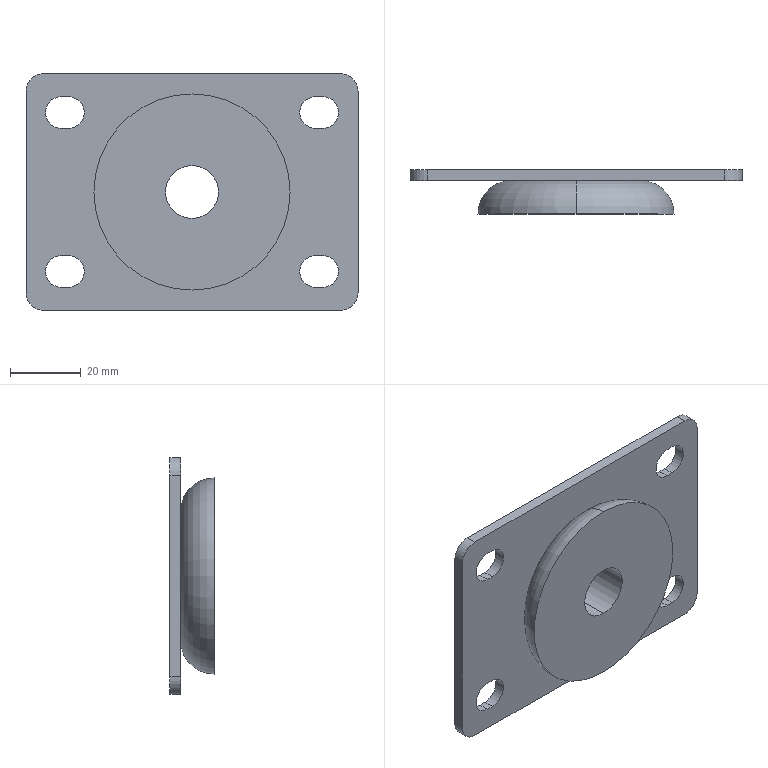Part | SolidWorks | features Cut 2, Extrusion 1, Fillet 1, Revolution 1 | 1 solid | 31 faces | box 94 x 12.5 x 67 mm | volume 35505 mm3 | plane 15 | cylinder 14 | torus 2 | commonest cylinder face diameters 9 x8 10 x4 15 x2
STEP:
#1=CARTESIAN_POINT('',(0.,3.,7.5));
#2=VERTEX_POINT('',#1);
#3=CARTESIAN_POINT('',(0.,3.,-7.5));
#4=VERTEX_POINT('',#3);
#5=CARTESIAN_POINT('',(0.,3.,0.));
#6=DIRECTION('',(0.,-1.,0.));
#7=DIRECTION('',(0.,0.,-1.));
#8=AXIS2_PLACEMENT_3D('',#5,#6,#7);
#9=CIRCLE('',#8,7.5);
#10=EDGE_CURVE('',#2,#4,#9,.T.);
#11=ORIENTED_EDGE('',*,*,#10,.F.);
#12=CARTESIAN_POINT('',(0.,-9.5,7.5));
#13=VERTEX_POINT('',#12);
#14=CARTESIAN_POINT('',(0.,3.,7.5));
#15=DIRECTION('',(0.,-1.,0.));
#16=VECTOR('',#15,1000.);
#17=LINE('',#14,#16);
#18=EDGE_CURVE('',#2,#13,#17,.T.);
#19=ORIENTED_EDGE('',*,*,#18,.T.);
#20=CARTESIAN_POINT('',(0.,-9.5,-7.5));
#21=VERTEX_POINT('',#20);
#22=CARTESIAN_POINT('',(0.,-9.5,0.));
#23=DIRECTION('',(0.,-1.,0.));
#24=DIRECTION('',(0.,0.,-1.));
#25=AXIS2_PLACEMENT_3D('',#22,#23,#24);
#26=CIRCLE('',#25,7.5);
#27=EDGE_CURVE('',#13,#21,#26,.T.);
#28=ORIENTED_EDGE('',*,*,#27,.T.);
#29=CARTESIAN_POINT('',(0.,3.,-7.5));
#30=DIRECTION('',(0.,-1.,0.));
#31=VECTOR('',#30,1000.);
#32=LINE('',#29,#31);
#33=EDGE_CURVE('',#4,#21,#32,.T.);
#34=ORIENTED_EDGE('',*,*,#33,.F.);
#35=EDGE_LOOP('',(#11,#19,#28,#34));
#36=FACE_OUTER_BOUND('',#35,.T.);
#37=CARTESIAN_POINT('',(0.,3.,0.));
#38=DIRECTION('',(0.,-1.,0.));
#39=DIRECTION('',(0.,0.,-1.));
#40=AXIS2_PLACEMENT_3D('',#37,#38,#39);
#41=CYLINDRICAL_SURFACE('',#40,7.5);
#42=ADVANCED_FACE('',(#36),#41,.F.);
#43=CARTESIAN_POINT('',(0.,-9.5,27.75));
#44=VERTEX_POINT('',#43);
#45=CARTESIAN_POINT('',(0.,-9.5,-27.75));
#46=VERTEX_POINT('',#45);
#47=CARTESIAN_POINT('',(0.,-9.5,0.));
#48=DIRECTION('',(0.,1.,0.));
#49=DIRECTION('',(0.,0.,1.));
#50=AXIS2_PLACEMENT_3D('',#47,#48,#49);
#51=CIRCLE('',#50,27.75);
#52=EDGE_CURVE('',#44,#46,#51,.T.);
#53=ORIENTED_EDGE('',*,*,#52,.T.);
#54=CARTESIAN_POINT('',(0.,0.,-18.25));
#55=VERTEX_POINT('',#54);
#56=CARTESIAN_POINT('',(0.,-9.5,-18.25));
#57=DIRECTION('',(1.,0.,0.));
#58=DIRECTION('',(0.,0.,-1.));
#59=AXIS2_PLACEMENT_3D('',#56,#57,#58);
#60=CIRCLE('',#59,9.5);
#61=EDGE_CURVE('',#46,#55,#60,.T.);
#62=ORIENTED_EDGE('',*,*,#61,.T.);
#63=CARTESIAN_POINT('',(0.,0.,18.25));
#64=VERTEX_POINT('',#63);
#65=CARTESIAN_POINT('',(0.,0.,0.));
#66=DIRECTION('',(0.,-1.,0.));
#67=DIRECTION('',(0.,0.,1.));
#68=AXIS2_PLACEMENT_3D('',#65,#66,#67);
#69=CIRCLE('',#68,18.25);
#70=EDGE_CURVE('',#55,#64,#69,.T.);
#71=ORIENTED_EDGE('',*,*,#70,.T.);
#72=CARTESIAN_POINT('',(0.,-9.5,18.25));
#73=DIRECTION('',(-1.,0.,0.));
#74=DIRECTION('',(0.,0.,1.));
#75=AXIS2_PLACEMENT_3D('',#72,#73,#74);
#76=CIRCLE('',#75,9.5);
#77=EDGE_CURVE('',#44,#64,#76,.T.);
#78=ORIENTED_EDGE('',*,*,#77,.F.);
#79=EDGE_LOOP('',(#53,#62,#71,#78));
#80=FACE_OUTER_BOUND('',#79,.T.);
#81=CARTESIAN_POINT('',(0.,-9.5,0.));
#82=DIRECTION('',(0.,1.,0.));
#83=DIRECTION('',(0.,0.,1.));
#84=AXIS2_PLACEMENT_3D('',#81,#82,#83);
#85=TOROIDAL_SURFACE('',#84,18.25,9.5);
#86=ADVANCED_FACE('',(#80),#85,.T.);
#87=CARTESIAN_POINT('',(-47.,0.,-28.5));
#88=VERTEX_POINT('',#87);
#89=CARTESIAN_POINT('',(-47.,0.,28.5));
#90=VERTEX_POINT('',#89);
#91=CARTESIAN_POINT('',(-47.,0.,-33.5));
#92=DIRECTION('',(0.,0.,1.));
#93=VECTOR('',#92,1000.);
#94=LINE('',#91,#93);
#95=EDGE_CURVE('',#88,#90,#94,.T.);
#96=ORIENTED_EDGE('',*,*,#95,.F.);
#97=CARTESIAN_POINT('',(-42.,0.,-33.5));
#98=VERTEX_POINT('',#97);
#99=CARTESIAN_POINT('',(-42.,0.,-28.5));
#100=DIRECTION('',(0.,-1.,0.));
#101=DIRECTION('',(0.,0.,1.));
#102=AXIS2_PLACEMENT_3D('',#99,#100,#101);
#103=CIRCLE('',#102,5.);
#104=EDGE_CURVE('',#88,#98,#103,.T.);
#105=ORIENTED_EDGE('',*,*,#104,.T.);
#106=CARTESIAN_POINT('',(42.,0.,-33.5));
#107=VERTEX_POINT('',#106);
#108=CARTESIAN_POINT('',(-47.,0.,-33.5));
#109=DIRECTION('',(-1.,0.,0.));
#110=VECTOR('',#109,1000.);
#111=LINE('',#108,#110);
#112=EDGE_CURVE('',#107,#98,#111,.T.);
#113=ORIENTED_EDGE('',*,*,#112,.F.);
#114=CARTESIAN_POINT('',(47.,0.,-28.5));
#115=VERTEX_POINT('',#114);
#116=CARTESIAN_POINT('',(42.,0.,-28.5));
#117=DIRECTION('',(0.,-1.,0.));
#118=DIRECTION('',(0.,0.,1.));
#119=AXIS2_PLACEMENT_3D('',#116,#117,#118);
#120=CIRCLE('',#119,5.);
#121=EDGE_CURVE('',#107,#115,#120,.T.);
#122=ORIENTED_EDGE('',*,*,#121,.T.);
#123=CARTESIAN_POINT('',(47.,0.,28.5));
#124=VERTEX_POINT('',#123);
#125=CARTESIAN_POINT('',(47.,0.,-33.5));
#126=DIRECTION('',(0.,0.,-1.));
#127=VECTOR('',#126,1000.);
#128=LINE('',#125,#127);
#129=EDGE_CURVE('',#124,#115,#128,.T.);
#130=ORIENTED_EDGE('',*,*,#129,.F.);
#131=CARTESIAN_POINT('',(42.,0.,33.5));
#132=VERTEX_POINT('',#131);
#133=CARTESIAN_POINT('',(42.,0.,28.5));
#134=DIRECTION('',(0.,-1.,0.));
#135=DIRECTION('',(0.,0.,1.));
#136=AXIS2_PLACEMENT_3D('',#133,#134,#135);
#137=CIRCLE('',#136,5.);
#138=EDGE_CURVE('',#124,#132,#137,.T.);
#139=ORIENTED_EDGE('',*,*,#138,.T.);
#140=CARTESIAN_POINT('',(-42.,0.,33.5));
#141=VERTEX_POINT('',#140);
#142=CARTESIAN_POINT('',(-47.,0.,33.5));
#143=DIRECTION('',(1.,0.,0.));
#144=VECTOR('',#143,1000.);
#145=LINE('',#142,#144);
#146=EDGE_CURVE('',#141,#132,#145,.T.);
#147=ORIENTED_EDGE('',*,*,#146,.F.);
#148=CARTESIAN_POINT('',(-42.,0.,28.5));
#149=DIRECTION('',(0.,-1.,0.));
#150=DIRECTION('',(0.,0.,1.));
#151=AXIS2_PLACEMENT_3D('',#148,#149,#150);
#152=CIRCLE('',#151,5.);
#153=EDGE_CURVE('',#141,#90,#152,.T.);
#154=ORIENTED_EDGE('',*,*,#153,.T.);
#155=EDGE_LOOP('',(#96,#105,#113,#122,#130,#139,#147,#154));
#156=FACE_OUTER_BOUND('',#155,.T.);
#157=CARTESIAN_POINT('',(35.,0.,27.));
#158=VERTEX_POINT('',#157);
#159=CARTESIAN_POINT('',(37.,0.,27.));
#160=VERTEX_POINT('',#159);
#161=CARTESIAN_POINT('',(35.,0.,27.));
#162=DIRECTION('',(1.,0.,0.));
#163=VECTOR('',#162,1000.);
#164=LINE('',#161,#163);
#165=EDGE_CURVE('',#158,#160,#164,.T.);
#166=ORIENTED_EDGE('',*,*,#165,.T.);
#167=CARTESIAN_POINT('',(37.,0.,18.));
#168=VERTEX_POINT('',#167);
#169=CARTESIAN_POINT('',(37.,0.,22.5));
#170=DIRECTION('',(0.,1.,0.));
#171=DIRECTION('',(0.,0.,-1.));
#172=AXIS2_PLACEMENT_3D('',#169,#170,#171);
#173=CIRCLE('',#172,4.5);
#174=EDGE_CURVE('',#160,#168,#173,.T.);
#175=ORIENTED_EDGE('',*,*,#174,.T.);
#176=CARTESIAN_POINT('',(35.,0.,18.));
#177=VERTEX_POINT('',#176);
#178=CARTESIAN_POINT('',(35.,0.,18.));
#179=DIRECTION('',(-1.,0.,0.));
#180=VECTOR('',#179,1000.);
#181=LINE('',#178,#180);
#182=EDGE_CURVE('',#168,#177,#181,.T.);
#183=ORIENTED_EDGE('',*,*,#182,.T.);
#184=CARTESIAN_POINT('',(35.,0.,22.5));
#185=DIRECTION('',(0.,1.,0.));
#186=DIRECTION('',(0.,0.,-1.));
#187=AXIS2_PLACEMENT_3D('',#184,#185,#186);
#188=CIRCLE('',#187,4.5);
#189=EDGE_CURVE('',#177,#158,#188,.T.);
#190=ORIENTED_EDGE('',*,*,#189,.T.);
#191=EDGE_LOOP('',(#166,#175,#183,#190));
#192=FACE_BOUND('',#191,.T.);
#193=CARTESIAN_POINT('',(-37.,0.,27.));
#194=VERTEX_POINT('',#193);
#195=CARTESIAN_POINT('',(-35.,0.,27.));
#196=VERTEX_POINT('',#195);
#197=CARTESIAN_POINT('',(-35.,0.,27.));
#198=DIRECTION('',(1.,0.,0.));
#199=VECTOR('',#198,1000.);
#200=LINE('',#197,#199);
#201=EDGE_CURVE('',#194,#196,#200,.T.);
#202=ORIENTED_EDGE('',*,*,#201,.T.);
#203=CARTESIAN_POINT('',(-35.,0.,18.));
#204=VERTEX_POINT('',#203);
#205=CARTESIAN_POINT('',(-35.,0.,22.5));
#206=DIRECTION('',(0.,1.,0.));
#207=DIRECTION('',(0.,0.,1.));
#208=AXIS2_PLACEMENT_3D('',#205,#206,#207);
#209=CIRCLE('',#208,4.5);
#210=EDGE_CURVE('',#196,#204,#209,.T.);
#211=ORIENTED_EDGE('',*,*,#210,.T.);
#212=CARTESIAN_POINT('',(-37.,0.,18.));
#213=VERTEX_POINT('',#212);
#214=CARTESIAN_POINT('',(-35.,0.,18.));
#215=DIRECTION('',(-1.,0.,0.));
#216=VECTOR('',#215,1000.);
#217=LINE('',#214,#216);
#218=EDGE_CURVE('',#204,#213,#217,.T.);
#219=ORIENTED_EDGE('',*,*,#218,.T.);
#220=CARTESIAN_POINT('',(-37.,0.,22.5));
#221=DIRECTION('',(0.,1.,0.));
#222=DIRECTION('',(0.,0.,1.));
#223=AXIS2_PLACEMENT_3D('',#220,#221,#222);
#224=CIRCLE('',#223,4.5);
#225=EDGE_CURVE('',#213,#194,#224,.T.);
#226=ORIENTED_EDGE('',*,*,#225,.T.);
#227=EDGE_LOOP('',(#202,#211,#219,#226));
#228=FACE_BOUND('',#227,.T.);
#229=CARTESIAN_POINT('',(37.,0.,-27.));
#230=VERTEX_POINT('',#229);
#231=CARTESIAN_POINT('',(35.,0.,-27.));
#232=VERTEX_POINT('',#231);
#233=CARTESIAN_POINT('',(35.,0.,-27.));
#234=DIRECTION('',(-1.,0.,0.));
#235=VECTOR('',#234,1000.);
#236=LINE('',#233,#235);
#237=EDGE_CURVE('',#230,#232,#236,.T.);
#238=ORIENTED_EDGE('',*,*,#237,.T.);
#239=CARTESIAN_POINT('',(35.,0.,-18.));
#240=VERTEX_POINT('',#239);
#241=CARTESIAN_POINT('',(35.,0.,-22.5));
#242=DIRECTION('',(0.,1.,0.));
#243=DIRECTION('',(0.,0.,1.));
#244=AXIS2_PLACEMENT_3D('',#241,#242,#243);
#245=CIRCLE('',#244,4.5);
#246=EDGE_CURVE('',#232,#240,#245,.T.);
#247=ORIENTED_EDGE('',*,*,#246,.T.);
#248=CARTESIAN_POINT('',(37.,0.,-18.));
#249=VERTEX_POINT('',#248);
#250=CARTESIAN_POINT('',(35.,0.,-18.));
#251=DIRECTION('',(1.,0.,0.));
#252=VECTOR('',#251,1000.);
#253=LINE('',#250,#252);
#254=EDGE_CURVE('',#240,#249,#253,.T.);
#255=ORIENTED_EDGE('',*,*,#254,.T.);
#256=CARTESIAN_POINT('',(37.,0.,-22.5));
#257=DIRECTION('',(0.,1.,0.));
#258=DIRECTION('',(0.,0.,1.));
#259=AXIS2_PLACEMENT_3D('',#256,#257,#258);
#260=CIRCLE('',#259,4.5);
#261=EDGE_CURVE('',#249,#230,#260,.T.);
#262=ORIENTED_EDGE('',*,*,#261,.T.);
#263=EDGE_LOOP('',(#238,#247,#255,#262));
#264=FACE_BOUND('',#263,.T.);
#265=CARTESIAN_POINT('',(-35.,0.,-27.));
#266=VERTEX_POINT('',#265);
#267=CARTESIAN_POINT('',(-37.,0.,-27.));
#268=VERTEX_POINT('',#267);
#269=CARTESIAN_POINT('',(-35.,0.,-27.));
#270=DIRECTION('',(-1.,0.,0.));
#271=VECTOR('',#270,1000.);
#272=LINE('',#269,#271);
#273=EDGE_CURVE('',#266,#268,#272,.T.);
#274=ORIENTED_EDGE('',*,*,#273,.T.);
#275=CARTESIAN_POINT('',(-37.,0.,-18.));
#276=VERTEX_POINT('',#275);
#277=CARTESIAN_POINT('',(-37.,0.,-22.5));
#278=DIRECTION('',(0.,1.,0.));
#279=DIRECTION('',(0.,0.,-1.));
#280=AXIS2_PLACEMENT_3D('',#277,#278,#279);
#281=CIRCLE('',#280,4.5);
#282=EDGE_CURVE('',#268,#276,#281,.T.);
#283=ORIENTED_EDGE('',*,*,#282,.T.);
#284=CARTESIAN_POINT('',(-35.,0.,-18.));
#285=VERTEX_POINT('',#284);
#286=CARTESIAN_POINT('',(-35.,0.,-18.));
#287=DIRECTION('',(1.,0.,0.));
#288=VECTOR('',#287,1000.);
#289=LINE('',#286,#288);
#290=EDGE_CURVE('',#276,#285,#289,.T.);
#291=ORIENTED_EDGE('',*,*,#290,.T.);
#292=CARTESIAN_POINT('',(-35.,0.,-22.5));
#293=DIRECTION('',(0.,1.,0.));
#294=DIRECTION('',(0.,0.,-1.));
#295=AXIS2_PLACEMENT_3D('',#292,#293,#294);
#296=CIRCLE('',#295,4.5);
#297=EDGE_CURVE('',#285,#266,#296,.T.);
#298=ORIENTED_EDGE('',*,*,#297,.T.);
#299=EDGE_LOOP('',(#274,#283,#291,#298));
#300=FACE_BOUND('',#299,.T.);
#301=CARTESIAN_POINT('',(0.,0.,0.));
#302=DIRECTION('',(0.,-1.,0.));
#303=DIRECTION('',(0.,0.,1.));
#304=AXIS2_PLACEMENT_3D('',#301,#302,#303);
#305=CIRCLE('',#304,18.25);
#306=EDGE_CURVE('',#64,#55,#305,.T.);
#307=ORIENTED_EDGE('',*,*,#306,.F.);
#308=ORIENTED_EDGE('',*,*,#70,.F.);
#309=EDGE_LOOP('',(#307,#308));
#310=FACE_BOUND('',#309,.T.);
#311=CARTESIAN_POINT('',(-47.,0.,33.5));
#312=DIRECTION('',(0.,1.,0.));
#313=DIRECTION('',(0.,0.,1.));
#314=AXIS2_PLACEMENT_3D('',#311,#312,#313);
#315=PLANE('',#314);
#316=ADVANCED_FACE('',(#156,#192,#228,#264,#300,#310),#315,.F.);
#317=CARTESIAN_POINT('',(-47.,3.,-28.5));
#318=VERTEX_POINT('',#317);
#319=CARTESIAN_POINT('',(-47.,3.,28.5));
#320=VERTEX_POINT('',#319);
#321=CARTESIAN_POINT('',(-47.,3.,-33.5));
#322=DIRECTION('',(0.,0.,1.));
#323=VECTOR('',#322,1000.);
#324=LINE('',#321,#323);
#325=EDGE_CURVE('',#318,#320,#324,.T.);
#326=ORIENTED_EDGE('',*,*,#325,.F.);
#327=CARTESIAN_POINT('',(-47.,3.,-28.5));
#328=DIRECTION('',(0.,-1.,0.));
#329=VECTOR('',#328,1000.);
#330=LINE('',#327,#329);
#331=EDGE_CURVE('',#318,#88,#330,.T.);
#332=ORIENTED_EDGE('',*,*,#331,.T.);
#333=ORIENTED_EDGE('',*,*,#95,.T.);
#334=CARTESIAN_POINT('',(-47.,3.,28.5));
#335=DIRECTION('',(0.,1.,0.));
#336=VECTOR('',#335,1000.);
#337=LINE('',#334,#336);
#338=EDGE_CURVE('',#90,#320,#337,.T.);
#339=ORIENTED_EDGE('',*,*,#338,.T.);
#340=EDGE_LOOP('',(#326,#332,#333,#339));
#341=FACE_OUTER_BOUND('',#340,.T.);
#342=CARTESIAN_POINT('',(-47.,3.,-33.5));
#343=DIRECTION('',(1.,0.,0.));
#344=DIRECTION('',(0.,0.,-1.));
#345=AXIS2_PLACEMENT_3D('',#342,#343,#344);
#346=PLANE('',#345);
#347=ADVANCED_FACE('',(#341),#346,.F.);
#348=CARTESIAN_POINT('',(-42.,3.,33.5));
#349=VERTEX_POINT('',#348);
#350=CARTESIAN_POINT('',(42.,3.,33.5));
#351=VERTEX_POINT('',#350);
#352=CARTESIAN_POINT('',(-47.,3.,33.5));
#353=DIRECTION('',(1.,0.,0.));
#354=VECTOR('',#353,1000.);
#355=LINE('',#352,#354);
#356=EDGE_CURVE('',#349,#351,#355,.T.);
#357=ORIENTED_EDGE('',*,*,#356,.F.);
#358=CARTESIAN_POINT('',(-42.,3.,33.5));
#359=DIRECTION('',(0.,-1.,0.));
#360=VECTOR('',#359,1000.);
#361=LINE('',#358,#360);
#362=EDGE_CURVE('',#349,#141,#361,.T.);
#363=ORIENTED_EDGE('',*,*,#362,.T.);
#364=ORIENTED_EDGE('',*,*,#146,.T.);
#365=CARTESIAN_POINT('',(42.,3.,33.5));
#366=DIRECTION('',(0.,1.,0.));
#367=VECTOR('',#366,1000.);
#368=LINE('',#365,#367);
#369=EDGE_CURVE('',#132,#351,#368,.T.);
#370=ORIENTED_EDGE('',*,*,#369,.T.);
#371=EDGE_LOOP('',(#357,#363,#364,#370));
#372=FACE_OUTER_BOUND('',#371,.T.);
#373=CARTESIAN_POINT('',(-47.,3.,33.5));
#374=DIRECTION('',(0.,0.,-1.));
#375=DIRECTION('',(-1.,0.,0.));
#376=AXIS2_PLACEMENT_3D('',#373,#374,#375);
#377=PLANE('',#376);
#378=ADVANCED_FACE('',(#372),#377,.F.);
#379=ORIENTED_EDGE('',*,*,#129,.T.);
#380=CARTESIAN_POINT('',(47.,3.,-28.5));
#381=VERTEX_POINT('',#380);
#382=CARTESIAN_POINT('',(47.,3.,-28.5));
#383=DIRECTION('',(0.,1.,0.));
#384=VECTOR('',#383,1000.);
#385=LINE('',#382,#384);
#386=EDGE_CURVE('',#115,#381,#385,.T.);
#387=ORIENTED_EDGE('',*,*,#386,.T.);
#388=CARTESIAN_POINT('',(47.,3.,28.5));
#389=VERTEX_POINT('',#388);
#390=CARTESIAN_POINT('',(47.,3.,-33.5));
#391=DIRECTION('',(0.,0.,-1.));
#392=VECTOR('',#391,1000.);
#393=LINE('',#390,#392);
#394=EDGE_CURVE('',#389,#381,#393,.T.);
#395=ORIENTED_EDGE('',*,*,#394,.F.);
#396=CARTESIAN_POINT('',(47.,3.,28.5));
#397=DIRECTION('',(0.,-1.,0.));
#398=VECTOR('',#397,1000.);
#399=LINE('',#396,#398);
#400=EDGE_CURVE('',#389,#124,#399,.T.);
#401=ORIENTED_EDGE('',*,*,#400,.T.);
#402=EDGE_LOOP('',(#379,#387,#395,#401));
#403=FACE_OUTER_BOUND('',#402,.T.);
#404=CARTESIAN_POINT('',(47.,3.,-33.5));
#405=DIRECTION('',(-1.,0.,0.));
#406=DIRECTION('',(0.,0.,1.));
#407=AXIS2_PLACEMENT_3D('',#404,#405,#406);
#408=PLANE('',#407);
#409=ADVANCED_FACE('',(#403),#408,.F.);
#410=ORIENTED_EDGE('',*,*,#112,.T.);
#411=CARTESIAN_POINT('',(-42.,3.,-33.5));
#412=VERTEX_POINT('',#411);
#413=CARTESIAN_POINT('',(-42.,3.,-33.5));
#414=DIRECTION('',(0.,1.,0.));
#415=VECTOR('',#414,1000.);
#416=LINE('',#413,#415);
#417=EDGE_CURVE('',#98,#412,#416,.T.);
#418=ORIENTED_EDGE('',*,*,#417,.T.);
#419=CARTESIAN_POINT('',(42.,3.,-33.5));
#420=VERTEX_POINT('',#419);
#421=CARTESIAN_POINT('',(-47.,3.,-33.5));
#422=DIRECTION('',(-1.,0.,0.));
#423=VECTOR('',#422,1000.);
#424=LINE('',#421,#423);
#425=EDGE_CURVE('',#420,#412,#424,.T.);
#426=ORIENTED_EDGE('',*,*,#425,.F.);
#427=CARTESIAN_POINT('',(42.,3.,-33.5));
#428=DIRECTION('',(0.,-1.,0.));
#429=VECTOR('',#428,1000.);
#430=LINE('',#427,#429);
#431=EDGE_CURVE('',#420,#107,#430,.T.);
#432=ORIENTED_EDGE('',*,*,#431,.T.);
#433=EDGE_LOOP('',(#410,#418,#426,#432));
#434=FACE_OUTER_BOUND('',#433,.T.);
#435=CARTESIAN_POINT('',(-47.,3.,-33.5));
#436=DIRECTION('',(0.,0.,1.));
#437=DIRECTION('',(1.,0.,0.));
#438=AXIS2_PLACEMENT_3D('',#435,#436,#437);
#439=PLANE('',#438);
#440=ADVANCED_FACE('',(#434),#439,.F.);
#441=CARTESIAN_POINT('',(0.,3.,0.));
#442=DIRECTION('',(0.,-1.,0.));
#443=DIRECTION('',(0.,0.,-1.));
#444=AXIS2_PLACEMENT_3D('',#441,#442,#443);
#445=CIRCLE('',#444,7.5);
#446=EDGE_CURVE('',#4,#2,#445,.T.);
#447=ORIENTED_EDGE('',*,*,#446,.T.);
#448=ORIENTED_EDGE('',*,*,#10,.T.);
#449=EDGE_LOOP('',(#447,#448));
#450=FACE_BOUND('',#449,.T.);
#451=CARTESIAN_POINT('',(-37.,3.,-27.));
#452=VERTEX_POINT('',#451);
#453=CARTESIAN_POINT('',(-37.,3.,-18.));
#454=VERTEX_POINT('',#453);
#455=CARTESIAN_POINT('',(-37.,3.,-22.5));
#456=DIRECTION('',(0.,1.,0.));
#457=DIRECTION('',(0.,0.,-1.));
#458=AXIS2_PLACEMENT_3D('',#455,#456,#457);
#459=CIRCLE('',#458,4.5);
#460=EDGE_CURVE('',#452,#454,#459,.T.);
#461=ORIENTED_EDGE('',*,*,#460,.F.);
#462=CARTESIAN_POINT('',(-35.,3.,-27.));
#463=VERTEX_POINT('',#462);
#464=CARTESIAN_POINT('',(-35.,3.,-27.));
#465=DIRECTION('',(-1.,0.,0.));
#466=VECTOR('',#465,1000.);
#467=LINE('',#464,#466);
#468=EDGE_CURVE('',#463,#452,#467,.T.);
#469=ORIENTED_EDGE('',*,*,#468,.F.);
#470=CARTESIAN_POINT('',(-35.,3.,-18.));
#471=VERTEX_POINT('',#470);
#472=CARTESIAN_POINT('',(-35.,3.,-22.5));
#473=DIRECTION('',(0.,1.,0.));
#474=DIRECTION('',(0.,0.,-1.));
#475=AXIS2_PLACEMENT_3D('',#472,#473,#474);
#476=CIRCLE('',#475,4.5);
#477=EDGE_CURVE('',#471,#463,#476,.T.);
#478=ORIENTED_EDGE('',*,*,#477,.F.);
#479=CARTESIAN_POINT('',(-35.,3.,-18.));
#480=DIRECTION('',(1.,0.,0.));
#481=VECTOR('',#480,1000.);
#482=LINE('',#479,#481);
#483=EDGE_CURVE('',#454,#471,#482,.T.);
#484=ORIENTED_EDGE('',*,*,#483,.F.);
#485=EDGE_LOOP('',(#461,#469,#478,#484));
#486=FACE_BOUND('',#485,.T.);
#487=CARTESIAN_POINT('',(35.,3.,-27.));
#488=VERTEX_POINT('',#487);
#489=CARTESIAN_POINT('',(35.,3.,-18.));
#490=VERTEX_POINT('',#489);
#491=CARTESIAN_POINT('',(35.,3.,-22.5));
#492=DIRECTION('',(0.,1.,0.));
#493=DIRECTION('',(0.,0.,1.));
#494=AXIS2_PLACEMENT_3D('',#491,#492,#493);
#495=CIRCLE('',#494,4.5);
#496=EDGE_CURVE('',#488,#490,#495,.T.);
#497=ORIENTED_EDGE('',*,*,#496,.F.);
#498=CARTESIAN_POINT('',(37.,3.,-27.));
#499=VERTEX_POINT('',#498);
#500=CARTESIAN_POINT('',(35.,3.,-27.));
#501=DIRECTION('',(-1.,0.,0.));
#502=VECTOR('',#501,1000.);
#503=LINE('',#500,#502);
#504=EDGE_CURVE('',#499,#488,#503,.T.);
#505=ORIENTED_EDGE('',*,*,#504,.F.);
#506=CARTESIAN_POINT('',(37.,3.,-18.));
#507=VERTEX_POINT('',#506);
#508=CARTESIAN_POINT('',(37.,3.,-22.5));
#509=DIRECTION('',(0.,1.,0.));
#510=DIRECTION('',(0.,0.,1.));
#511=AXIS2_PLACEMENT_3D('',#508,#509,#510);
#512=CIRCLE('',#511,4.5);
#513=EDGE_CURVE('',#507,#499,#512,.T.);
#514=ORIENTED_EDGE('',*,*,#513,.F.);
#515=CARTESIAN_POINT('',(35.,3.,-18.));
#516=DIRECTION('',(1.,0.,0.));
#517=VECTOR('',#516,1000.);
#518=LINE('',#515,#517);
#519=EDGE_CURVE('',#490,#507,#518,.T.);
#520=ORIENTED_EDGE('',*,*,#519,.F.);
#521=EDGE_LOOP('',(#497,#505,#514,#520));
#522=FACE_BOUND('',#521,.T.);
#523=CARTESIAN_POINT('',(-35.,3.,27.));
#524=VERTEX_POINT('',#523);
#525=CARTESIAN_POINT('',(-35.,3.,18.));
#526=VERTEX_POINT('',#525);
#527=CARTESIAN_POINT('',(-35.,3.,22.5));
#528=DIRECTION('',(0.,1.,0.));
#529=DIRECTION('',(0.,0.,1.));
#530=AXIS2_PLACEMENT_3D('',#527,#528,#529);
#531=CIRCLE('',#530,4.5);
#532=EDGE_CURVE('',#524,#526,#531,.T.);
#533=ORIENTED_EDGE('',*,*,#532,.F.);
#534=CARTESIAN_POINT('',(-37.,3.,27.));
#535=VERTEX_POINT('',#534);
#536=CARTESIAN_POINT('',(-35.,3.,27.));
#537=DIRECTION('',(1.,0.,0.));
#538=VECTOR('',#537,1000.);
#539=LINE('',#536,#538);
#540=EDGE_CURVE('',#535,#524,#539,.T.);
#541=ORIENTED_EDGE('',*,*,#540,.F.);
#542=CARTESIAN_POINT('',(-37.,3.,18.));
#543=VERTEX_POINT('',#542);
#544=CARTESIAN_POINT('',(-37.,3.,22.5));
#545=DIRECTION('',(0.,1.,0.));
#546=DIRECTION('',(0.,0.,1.));
#547=AXIS2_PLACEMENT_3D('',#544,#545,#546);
#548=CIRCLE('',#547,4.5);
#549=EDGE_CURVE('',#543,#535,#548,.T.);
#550=ORIENTED_EDGE('',*,*,#549,.F.);
#551=CARTESIAN_POINT('',(-35.,3.,18.));
#552=DIRECTION('',(-1.,0.,0.));
#553=VECTOR('',#552,1000.);
#554=LINE('',#551,#553);
#555=EDGE_CURVE('',#526,#543,#554,.T.);
#556=ORIENTED_EDGE('',*,*,#555,.F.);
#557=EDGE_LOOP('',(#533,#541,#550,#556));
#558=FACE_BOUND('',#557,.T.);
#559=CARTESIAN_POINT('',(37.,3.,27.));
#560=VERTEX_POINT('',#559);
#561=CARTESIAN_POINT('',(37.,3.,18.));
#562=VERTEX_POINT('',#561);
#563=CARTESIAN_POINT('',(37.,3.,22.5));
#564=DIRECTION('',(0.,1.,0.));
#565=DIRECTION('',(0.,0.,-1.));
#566=AXIS2_PLACEMENT_3D('',#563,#564,#565);
#567=CIRCLE('',#566,4.5);
#568=EDGE_CURVE('',#560,#562,#567,.T.);
#569=ORIENTED_EDGE('',*,*,#568,.F.);
#570=CARTESIAN_POINT('',(35.,3.,27.));
#571=VERTEX_POINT('',#570);
#572=CARTESIAN_POINT('',(35.,3.,27.));
#573=DIRECTION('',(1.,0.,0.));
#574=VECTOR('',#573,1000.);
#575=LINE('',#572,#574);
#576=EDGE_CURVE('',#571,#560,#575,.T.);
#577=ORIENTED_EDGE('',*,*,#576,.F.);
#578=CARTESIAN_POINT('',(35.,3.,18.));
#579=VERTEX_POINT('',#578);
#580=CARTESIAN_POINT('',(35.,3.,22.5));
#581=DIRECTION('',(0.,1.,0.));
#582=DIRECTION('',(0.,0.,-1.));
#583=AXIS2_PLACEMENT_3D('',#580,#581,#582);
#584=CIRCLE('',#583,4.5);
#585=EDGE_CURVE('',#579,#571,#584,.T.);
#586=ORIENTED_EDGE('',*,*,#585,.F.);
#587=CARTESIAN_POINT('',(35.,3.,18.));
#588=DIRECTION('',(-1.,0.,0.));
#589=VECTOR('',#588,1000.);
#590=LINE('',#587,#589);
#591=EDGE_CURVE('',#562,#579,#590,.T.);
#592=ORIENTED_EDGE('',*,*,#591,.F.);
#593=EDGE_LOOP('',(#569,#577,#586,#592));
#594=FACE_BOUND('',#593,.T.);
#595=ORIENTED_EDGE('',*,*,#425,.T.);
#596=CARTESIAN_POINT('',(-42.,3.,-28.5));
#597=DIRECTION('',(0.,1.,0.));
#598=DIRECTION('',(0.,0.,1.));
#599=AXIS2_PLACEMENT_3D('',#596,#597,#598);
#600=CIRCLE('',#599,5.);
#601=EDGE_CURVE('',#412,#318,#600,.T.);
#602=ORIENTED_EDGE('',*,*,#601,.T.);
#603=ORIENTED_EDGE('',*,*,#325,.T.);
#604=CARTESIAN_POINT('',(-42.,3.,28.5));
#605=DIRECTION('',(0.,1.,0.));
#606=DIRECTION('',(0.,0.,1.));
#607=AXIS2_PLACEMENT_3D('',#604,#605,#606);
#608=CIRCLE('',#607,5.);
#609=EDGE_CURVE('',#320,#349,#608,.T.);
#610=ORIENTED_EDGE('',*,*,#609,.T.);
#611=ORIENTED_EDGE('',*,*,#356,.T.);
#612=CARTESIAN_POINT('',(42.,3.,28.5));
#613=DIRECTION('',(0.,1.,0.));
#614=DIRECTION('',(0.,0.,1.));
#615=AXIS2_PLACEMENT_3D('',#612,#613,#614);
#616=CIRCLE('',#615,5.);
#617=EDGE_CURVE('',#351,#389,#616,.T.);
#618=ORIENTED_EDGE('',*,*,#617,.T.);
#619=ORIENTED_EDGE('',*,*,#394,.T.);
#620=CARTESIAN_POINT('',(42.,3.,-28.5));
#621=DIRECTION('',(0.,1.,0.));
#622=DIRECTION('',(0.,0.,1.));
#623=AXIS2_PLACEMENT_3D('',#620,#621,#622);
#624=CIRCLE('',#623,5.);
#625=EDGE_CURVE('',#381,#420,#624,.T.);
#626=ORIENTED_EDGE('',*,*,#625,.T.);
#627=EDGE_LOOP('',(#595,#602,#603,#610,#611,#618,#619,#626));
#628=FACE_OUTER_BOUND('',#627,.T.);
#629=CARTESIAN_POINT('',(-47.,3.,33.5));
#630=DIRECTION('',(0.,1.,0.));
#631=DIRECTION('',(0.,0.,1.));
#632=AXIS2_PLACEMENT_3D('',#629,#630,#631);
#633=PLANE('',#632);
#634=ADVANCED_FACE('',(#450,#486,#522,#558,#594,#628),#633,.T.);
#635=ORIENTED_EDGE('',*,*,#601,.F.);
#636=ORIENTED_EDGE('',*,*,#417,.F.);
#637=ORIENTED_EDGE('',*,*,#104,.F.);
#638=ORIENTED_EDGE('',*,*,#331,.F.);
#639=EDGE_LOOP('',(#635,#636,#637,#638));
#640=FACE_OUTER_BOUND('',#639,.T.);
#641=CARTESIAN_POINT('',(-42.,3.,-28.5));
#642=DIRECTION('',(0.,-1.,0.));
#643=DIRECTION('',(0.,0.,-1.));
#644=AXIS2_PLACEMENT_3D('',#641,#642,#643);
#645=CYLINDRICAL_SURFACE('',#644,5.);
#646=ADVANCED_FACE('',(#640),#645,.T.);
#647=ORIENTED_EDGE('',*,*,#609,.F.);
#648=ORIENTED_EDGE('',*,*,#338,.F.);
#649=ORIENTED_EDGE('',*,*,#153,.F.);
#650=ORIENTED_EDGE('',*,*,#362,.F.);
#651=EDGE_LOOP('',(#647,#648,#649,#650));
#652=FACE_OUTER_BOUND('',#651,.T.);
#653=CARTESIAN_POINT('',(-42.,3.,28.5));
#654=DIRECTION('',(0.,-1.,0.));
#655=DIRECTION('',(0.,0.,-1.));
#656=AXIS2_PLACEMENT_3D('',#653,#654,#655);
#657=CYLINDRICAL_SURFACE('',#656,5.);
#658=ADVANCED_FACE('',(#652),#657,.T.);
#659=ORIENTED_EDGE('',*,*,#625,.F.);
#660=ORIENTED_EDGE('',*,*,#386,.F.);
#661=ORIENTED_EDGE('',*,*,#121,.F.);
#662=ORIENTED_EDGE('',*,*,#431,.F.);
#663=EDGE_LOOP('',(#659,#660,#661,#662));
#664=FACE_OUTER_BOUND('',#663,.T.);
#665=CARTESIAN_POINT('',(42.,3.,-28.5));
#666=DIRECTION('',(0.,-1.,0.));
#667=DIRECTION('',(0.,0.,-1.));
#668=AXIS2_PLACEMENT_3D('',#665,#666,#667);
#669=CYLINDRICAL_SURFACE('',#668,5.);
#670=ADVANCED_FACE('',(#664),#669,.T.);
#671=ORIENTED_EDGE('',*,*,#617,.F.);
#672=ORIENTED_EDGE('',*,*,#369,.F.);
#673=ORIENTED_EDGE('',*,*,#138,.F.);
#674=ORIENTED_EDGE('',*,*,#400,.F.);
#675=EDGE_LOOP('',(#671,#672,#673,#674));
#676=FACE_OUTER_BOUND('',#675,.T.);
#677=CARTESIAN_POINT('',(42.,3.,28.5));
#678=DIRECTION('',(0.,-1.,0.));
#679=DIRECTION('',(0.,0.,-1.));
#680=AXIS2_PLACEMENT_3D('',#677,#678,#679);
#681=CYLINDRICAL_SURFACE('',#680,5.);
#682=ADVANCED_FACE('',(#676),#681,.T.);
#683=ORIENTED_EDGE('',*,*,#568,.T.);
#684=CARTESIAN_POINT('',(37.,0.,18.));
#685=DIRECTION('',(0.,1.,0.));
#686=VECTOR('',#685,1000.);
#687=LINE('',#684,#686);
#688=EDGE_CURVE('',#168,#562,#687,.T.);
#689=ORIENTED_EDGE('',*,*,#688,.F.);
#690=ORIENTED_EDGE('',*,*,#174,.F.);
#691=CARTESIAN_POINT('',(37.,0.,27.));
#692=DIRECTION('',(0.,1.,0.));
#693=VECTOR('',#692,1000.);
#694=LINE('',#691,#693);
#695=EDGE_CURVE('',#160,#560,#694,.T.);
#696=ORIENTED_EDGE('',*,*,#695,.T.);
#697=EDGE_LOOP('',(#683,#689,#690,#696));
#698=FACE_OUTER_BOUND('',#697,.T.);
#699=CARTESIAN_POINT('',(37.,0.,22.5));
#700=DIRECTION('',(0.,1.,0.));
#701=DIRECTION('',(0.,0.,1.));
#702=AXIS2_PLACEMENT_3D('',#699,#700,#701);
#703=CYLINDRICAL_SURFACE('',#702,4.5);
#704=ADVANCED_FACE('',(#698),#703,.F.);
#705=ORIENTED_EDGE('',*,*,#576,.T.);
#706=ORIENTED_EDGE('',*,*,#695,.F.);
#707=ORIENTED_EDGE('',*,*,#165,.F.);
#708=CARTESIAN_POINT('',(35.,0.,27.));
#709=DIRECTION('',(0.,1.,0.));
#710=VECTOR('',#709,1000.);
#711=LINE('',#708,#710);
#712=EDGE_CURVE('',#158,#571,#711,.T.);
#713=ORIENTED_EDGE('',*,*,#712,.T.);
#714=EDGE_LOOP('',(#705,#706,#707,#713));
#715=FACE_OUTER_BOUND('',#714,.T.);
#716=CARTESIAN_POINT('',(35.,0.,27.));
#717=DIRECTION('',(0.,0.,1.));
#718=DIRECTION('',(1.,0.,0.));
#719=AXIS2_PLACEMENT_3D('',#716,#717,#718);
#720=PLANE('',#719);
#721=ADVANCED_FACE('',(#715),#720,.F.);
#722=ORIENTED_EDGE('',*,*,#585,.T.);
#723=ORIENTED_EDGE('',*,*,#712,.F.);
#724=ORIENTED_EDGE('',*,*,#189,.F.);
#725=CARTESIAN_POINT('',(35.,0.,18.));
#726=DIRECTION('',(0.,1.,0.));
#727=VECTOR('',#726,1000.);
#728=LINE('',#725,#727);
#729=EDGE_CURVE('',#177,#579,#728,.T.);
#730=ORIENTED_EDGE('',*,*,#729,.T.);
#731=EDGE_LOOP('',(#722,#723,#724,#730));
#732=FACE_OUTER_BOUND('',#731,.T.);
#733=CARTESIAN_POINT('',(35.,0.,22.5));
#734=DIRECTION('',(0.,1.,0.));
#735=DIRECTION('',(0.,0.,1.));
#736=AXIS2_PLACEMENT_3D('',#733,#734,#735);
#737=CYLINDRICAL_SURFACE('',#736,4.5);
#738=ADVANCED_FACE('',(#732),#737,.F.);
#739=ORIENTED_EDGE('',*,*,#591,.T.);
#740=ORIENTED_EDGE('',*,*,#729,.F.);
#741=ORIENTED_EDGE('',*,*,#182,.F.);
#742=ORIENTED_EDGE('',*,*,#688,.T.);
#743=EDGE_LOOP('',(#739,#740,#741,#742));
#744=FACE_OUTER_BOUND('',#743,.T.);
#745=CARTESIAN_POINT('',(35.,0.,18.));
#746=DIRECTION('',(0.,0.,-1.));
#747=DIRECTION('',(-1.,0.,0.));
#748=AXIS2_PLACEMENT_3D('',#745,#746,#747);
#749=PLANE('',#748);
#750=ADVANCED_FACE('',(#744),#749,.F.);
#751=ORIENTED_EDGE('',*,*,#532,.T.);
#752=CARTESIAN_POINT('',(-35.,0.,18.));
#753=DIRECTION('',(0.,1.,0.));
#754=VECTOR('',#753,1000.);
#755=LINE('',#752,#754);
#756=EDGE_CURVE('',#204,#526,#755,.T.);
#757=ORIENTED_EDGE('',*,*,#756,.F.);
#758=ORIENTED_EDGE('',*,*,#210,.F.);
#759=CARTESIAN_POINT('',(-35.,0.,27.));
#760=DIRECTION('',(0.,1.,0.));
#761=VECTOR('',#760,1000.);
#762=LINE('',#759,#761);
#763=EDGE_CURVE('',#196,#524,#762,.T.);
#764=ORIENTED_EDGE('',*,*,#763,.T.);
#765=EDGE_LOOP('',(#751,#757,#758,#764));
#766=FACE_OUTER_BOUND('',#765,.T.);
#767=CARTESIAN_POINT('',(-35.,0.,22.5));
#768=DIRECTION('',(0.,1.,0.));
#769=DIRECTION('',(0.,0.,1.));
#770=AXIS2_PLACEMENT_3D('',#767,#768,#769);
#771=CYLINDRICAL_SURFACE('',#770,4.5);
#772=ADVANCED_FACE('',(#766),#771,.F.);
#773=ORIENTED_EDGE('',*,*,#540,.T.);
#774=ORIENTED_EDGE('',*,*,#763,.F.);
#775=ORIENTED_EDGE('',*,*,#201,.F.);
#776=CARTESIAN_POINT('',(-37.,0.,27.));
#777=DIRECTION('',(0.,1.,0.));
#778=VECTOR('',#777,1000.);
#779=LINE('',#776,#778);
#780=EDGE_CURVE('',#194,#535,#779,.T.);
#781=ORIENTED_EDGE('',*,*,#780,.T.);
#782=EDGE_LOOP('',(#773,#774,#775,#781));
#783=FACE_OUTER_BOUND('',#782,.T.);
#784=CARTESIAN_POINT('',(-35.,0.,27.));
#785=DIRECTION('',(0.,0.,1.));
#786=DIRECTION('',(1.,0.,0.));
#787=AXIS2_PLACEMENT_3D('',#784,#785,#786);
#788=PLANE('',#787);
#789=ADVANCED_FACE('',(#783),#788,.F.);
#790=ORIENTED_EDGE('',*,*,#549,.T.);
#791=ORIENTED_EDGE('',*,*,#780,.F.);
#792=ORIENTED_EDGE('',*,*,#225,.F.);
#793=CARTESIAN_POINT('',(-37.,0.,18.));
#794=DIRECTION('',(0.,1.,0.));
#795=VECTOR('',#794,1000.);
#796=LINE('',#793,#795);
#797=EDGE_CURVE('',#213,#543,#796,.T.);
#798=ORIENTED_EDGE('',*,*,#797,.T.);
#799=EDGE_LOOP('',(#790,#791,#792,#798));
#800=FACE_OUTER_BOUND('',#799,.T.);
#801=CARTESIAN_POINT('',(-37.,0.,22.5));
#802=DIRECTION('',(0.,1.,0.));
#803=DIRECTION('',(0.,0.,1.));
#804=AXIS2_PLACEMENT_3D('',#801,#802,#803);
#805=CYLINDRICAL_SURFACE('',#804,4.5);
#806=ADVANCED_FACE('',(#800),#805,.F.);
#807=ORIENTED_EDGE('',*,*,#555,.T.);
#808=ORIENTED_EDGE('',*,*,#797,.F.);
#809=ORIENTED_EDGE('',*,*,#218,.F.);
#810=ORIENTED_EDGE('',*,*,#756,.T.);
#811=EDGE_LOOP('',(#807,#808,#809,#810));
#812=FACE_OUTER_BOUND('',#811,.T.);
#813=CARTESIAN_POINT('',(-35.,0.,18.));
#814=DIRECTION('',(0.,0.,-1.));
#815=DIRECTION('',(-1.,0.,0.));
#816=AXIS2_PLACEMENT_3D('',#813,#814,#815);
#817=PLANE('',#816);
#818=ADVANCED_FACE('',(#812),#817,.F.);
#819=ORIENTED_EDGE('',*,*,#496,.T.);
#820=CARTESIAN_POINT('',(35.,0.,-18.));
#821=DIRECTION('',(0.,1.,0.));
#822=VECTOR('',#821,1000.);
#823=LINE('',#820,#822);
#824=EDGE_CURVE('',#240,#490,#823,.T.);
#825=ORIENTED_EDGE('',*,*,#824,.F.);
#826=ORIENTED_EDGE('',*,*,#246,.F.);
#827=CARTESIAN_POINT('',(35.,0.,-27.));
#828=DIRECTION('',(0.,1.,0.));
#829=VECTOR('',#828,1000.);
#830=LINE('',#827,#829);
#831=EDGE_CURVE('',#232,#488,#830,.T.);
#832=ORIENTED_EDGE('',*,*,#831,.T.);
#833=EDGE_LOOP('',(#819,#825,#826,#832));
#834=FACE_OUTER_BOUND('',#833,.T.);
#835=CARTESIAN_POINT('',(35.,0.,-22.5));
#836=DIRECTION('',(0.,1.,0.));
#837=DIRECTION('',(0.,0.,1.));
#838=AXIS2_PLACEMENT_3D('',#835,#836,#837);
#839=CYLINDRICAL_SURFACE('',#838,4.5);
#840=ADVANCED_FACE('',(#834),#839,.F.);
#841=ORIENTED_EDGE('',*,*,#504,.T.);
#842=ORIENTED_EDGE('',*,*,#831,.F.);
#843=ORIENTED_EDGE('',*,*,#237,.F.);
#844=CARTESIAN_POINT('',(37.,0.,-27.));
#845=DIRECTION('',(0.,1.,0.));
#846=VECTOR('',#845,1000.);
#847=LINE('',#844,#846);
#848=EDGE_CURVE('',#230,#499,#847,.T.);
#849=ORIENTED_EDGE('',*,*,#848,.T.);
#850=EDGE_LOOP('',(#841,#842,#843,#849));
#851=FACE_OUTER_BOUND('',#850,.T.);
#852=CARTESIAN_POINT('',(35.,0.,-27.));
#853=DIRECTION('',(0.,0.,-1.));
#854=DIRECTION('',(-1.,0.,0.));
#855=AXIS2_PLACEMENT_3D('',#852,#853,#854);
#856=PLANE('',#855);
#857=ADVANCED_FACE('',(#851),#856,.F.);
#858=ORIENTED_EDGE('',*,*,#513,.T.);
#859=ORIENTED_EDGE('',*,*,#848,.F.);
#860=ORIENTED_EDGE('',*,*,#261,.F.);
#861=CARTESIAN_POINT('',(37.,0.,-18.));
#862=DIRECTION('',(0.,1.,0.));
#863=VECTOR('',#862,1000.);
#864=LINE('',#861,#863);
#865=EDGE_CURVE('',#249,#507,#864,.T.);
#866=ORIENTED_EDGE('',*,*,#865,.T.);
#867=EDGE_LOOP('',(#858,#859,#860,#866));
#868=FACE_OUTER_BOUND('',#867,.T.);
#869=CARTESIAN_POINT('',(37.,0.,-22.5));
#870=DIRECTION('',(0.,1.,0.));
#871=DIRECTION('',(0.,0.,1.));
#872=AXIS2_PLACEMENT_3D('',#869,#870,#871);
#873=CYLINDRICAL_SURFACE('',#872,4.5);
#874=ADVANCED_FACE('',(#868),#873,.F.);
#875=ORIENTED_EDGE('',*,*,#519,.T.);
#876=ORIENTED_EDGE('',*,*,#865,.F.);
#877=ORIENTED_EDGE('',*,*,#254,.F.);
#878=ORIENTED_EDGE('',*,*,#824,.T.);
#879=EDGE_LOOP('',(#875,#876,#877,#878));
#880=FACE_OUTER_BOUND('',#879,.T.);
#881=CARTESIAN_POINT('',(35.,0.,-18.));
#882=DIRECTION('',(0.,0.,1.));
#883=DIRECTION('',(1.,0.,0.));
#884=AXIS2_PLACEMENT_3D('',#881,#882,#883);
#885=PLANE('',#884);
#886=ADVANCED_FACE('',(#880),#885,.F.);
#887=ORIENTED_EDGE('',*,*,#460,.T.);
#888=CARTESIAN_POINT('',(-37.,0.,-18.));
#889=DIRECTION('',(0.,1.,0.));
#890=VECTOR('',#889,1000.);
#891=LINE('',#888,#890);
#892=EDGE_CURVE('',#276,#454,#891,.T.);
#893=ORIENTED_EDGE('',*,*,#892,.F.);
#894=ORIENTED_EDGE('',*,*,#282,.F.);
#895=CARTESIAN_POINT('',(-37.,0.,-27.));
#896=DIRECTION('',(0.,1.,0.));
#897=VECTOR('',#896,1000.);
#898=LINE('',#895,#897);
#899=EDGE_CURVE('',#268,#452,#898,.T.);
#900=ORIENTED_EDGE('',*,*,#899,.T.);
#901=EDGE_LOOP('',(#887,#893,#894,#900));
#902=FACE_OUTER_BOUND('',#901,.T.);
#903=CARTESIAN_POINT('',(-37.,0.,-22.5));
#904=DIRECTION('',(0.,1.,0.));
#905=DIRECTION('',(0.,0.,1.));
#906=AXIS2_PLACEMENT_3D('',#903,#904,#905);
#907=CYLINDRICAL_SURFACE('',#906,4.5);
#908=ADVANCED_FACE('',(#902),#907,.F.);
#909=ORIENTED_EDGE('',*,*,#468,.T.);
#910=ORIENTED_EDGE('',*,*,#899,.F.);
#911=ORIENTED_EDGE('',*,*,#273,.F.);
#912=CARTESIAN_POINT('',(-35.,0.,-27.));
#913=DIRECTION('',(0.,1.,0.));
#914=VECTOR('',#913,1000.);
#915=LINE('',#912,#914);
#916=EDGE_CURVE('',#266,#463,#915,.T.);
#917=ORIENTED_EDGE('',*,*,#916,.T.);
#918=EDGE_LOOP('',(#909,#910,#911,#917));
#919=FACE_OUTER_BOUND('',#918,.T.);
#920=CARTESIAN_POINT('',(-35.,0.,-27.));
#921=DIRECTION('',(0.,0.,-1.));
#922=DIRECTION('',(-1.,0.,0.));
#923=AXIS2_PLACEMENT_3D('',#920,#921,#922);
#924=PLANE('',#923);
#925=ADVANCED_FACE('',(#919),#924,.F.);
#926=ORIENTED_EDGE('',*,*,#477,.T.);
#927=ORIENTED_EDGE('',*,*,#916,.F.);
#928=ORIENTED_EDGE('',*,*,#297,.F.);
#929=CARTESIAN_POINT('',(-35.,0.,-18.));
#930=DIRECTION('',(0.,1.,0.));
#931=VECTOR('',#930,1000.);
#932=LINE('',#929,#931);
#933=EDGE_CURVE('',#285,#471,#932,.T.);
#934=ORIENTED_EDGE('',*,*,#933,.T.);
#935=EDGE_LOOP('',(#926,#927,#928,#934));
#936=FACE_OUTER_BOUND('',#935,.T.);
#937=CARTESIAN_POINT('',(-35.,0.,-22.5));
#938=DIRECTION('',(0.,1.,0.));
#939=DIRECTION('',(0.,0.,1.));
#940=AXIS2_PLACEMENT_3D('',#937,#938,#939);
#941=CYLINDRICAL_SURFACE('',#940,4.5);
#942=ADVANCED_FACE('',(#936),#941,.F.);
#943=ORIENTED_EDGE('',*,*,#483,.T.);
#944=ORIENTED_EDGE('',*,*,#933,.F.);
#945=ORIENTED_EDGE('',*,*,#290,.F.);
#946=ORIENTED_EDGE('',*,*,#892,.T.);
#947=EDGE_LOOP('',(#943,#944,#945,#946));
#948=FACE_OUTER_BOUND('',#947,.T.);
#949=CARTESIAN_POINT('',(-35.,0.,-18.));
#950=DIRECTION('',(0.,0.,1.));
#951=DIRECTION('',(1.,0.,0.));
#952=AXIS2_PLACEMENT_3D('',#949,#950,#951);
#953=PLANE('',#952);
#954=ADVANCED_FACE('',(#948),#953,.F.);
#955=ORIENTED_EDGE('',*,*,#61,.F.);
#956=CARTESIAN_POINT('',(0.,-9.5,0.));
#957=DIRECTION('',(0.,1.,0.));
#958=DIRECTION('',(0.,0.,1.));
#959=AXIS2_PLACEMENT_3D('',#956,#957,#958);
#960=CIRCLE('',#959,27.75);
#961=EDGE_CURVE('',#46,#44,#960,.T.);
#962=ORIENTED_EDGE('',*,*,#961,.T.);
#963=ORIENTED_EDGE('',*,*,#77,.T.);
#964=ORIENTED_EDGE('',*,*,#306,.T.);
#965=EDGE_LOOP('',(#955,#962,#963,#964));
#966=FACE_OUTER_BOUND('',#965,.T.);
#967=CARTESIAN_POINT('',(0.,-9.5,0.));
#968=DIRECTION('',(0.,1.,0.));
#969=DIRECTION('',(0.,0.,1.));
#970=AXIS2_PLACEMENT_3D('',#967,#968,#969);
#971=TOROIDAL_SURFACE('',#970,18.25,9.5);
#972=ADVANCED_FACE('',(#966),#971,.T.);
#973=CARTESIAN_POINT('',(0.,-9.5,0.));
#974=DIRECTION('',(0.,-1.,0.));
#975=DIRECTION('',(0.,0.,-1.));
#976=AXIS2_PLACEMENT_3D('',#973,#974,#975);
#977=CIRCLE('',#976,7.5);
#978=EDGE_CURVE('',#21,#13,#977,.T.);
#979=ORIENTED_EDGE('',*,*,#978,.F.);
#980=ORIENTED_EDGE('',*,*,#27,.F.);
#981=EDGE_LOOP('',(#979,#980));
#982=FACE_BOUND('',#981,.T.);
#983=ORIENTED_EDGE('',*,*,#52,.F.);
#984=ORIENTED_EDGE('',*,*,#961,.F.);
#985=EDGE_LOOP('',(#983,#984));
#986=FACE_OUTER_BOUND('',#985,.T.);
#987=CARTESIAN_POINT('',(0.,-9.5,0.));
#988=DIRECTION('',(0.,1.,0.));
#989=DIRECTION('',(0.,0.,1.));
#990=AXIS2_PLACEMENT_3D('',#987,#988,#989);
#991=PLANE('',#990);
#992=ADVANCED_FACE('',(#982,#986),#991,.F.);
#993=ORIENTED_EDGE('',*,*,#18,.F.);
#994=ORIENTED_EDGE('',*,*,#446,.F.);
#995=ORIENTED_EDGE('',*,*,#33,.T.);
#996=ORIENTED_EDGE('',*,*,#978,.T.);
#997=EDGE_LOOP('',(#993,#994,#995,#996));
#998=FACE_OUTER_BOUND('',#997,.T.);
#999=CARTESIAN_POINT('',(0.,3.,0.));
#1000=DIRECTION('',(0.,-1.,0.));
#1001=DIRECTION('',(0.,0.,-1.));
#1002=AXIS2_PLACEMENT_3D('',#999,#1000,#1001);
#1003=CYLINDRICAL_SURFACE('',#1002,7.5);
#1004=ADVANCED_FACE('',(#998),#1003,.F.);
#1005=CLOSED_SHELL('',(#42,#86,#316,#347,#378,#409,#440,#634,#646,#658,#670,#682,#704,#721,#738,#750,#772,#789,#806,#818,#840,#857,#874,#886,#908,#925,#942,#954,#972,#992,#1004));
#1006=MANIFOLD_SOLID_BREP('',#1005);
#1007=CARTESIAN_POINT('',(0.,0.,0.));
#1008=DIRECTION('',(0.,0.,1.));
#1009=DIRECTION('',(1.,0.,0.));
#1010=AXIS2_PLACEMENT_3D('',#1007,#1008,#1009);
#1011=(LENGTH_UNIT()NAMED_UNIT(*)SI_UNIT(.MILLI.,.METRE.));
#1012=UNCERTAINTY_MEASURE_WITH_UNIT(LENGTH_MEASURE(0.00001),#1011,'','');
#1013=(NAMED_UNIT(*)PLANE_ANGLE_UNIT()SI_UNIT($,.RADIAN.));
#1014=(NAMED_UNIT(*)SI_UNIT($,.STERADIAN.)SOLID_ANGLE_UNIT());
#1015=(GEOMETRIC_REPRESENTATION_CONTEXT(3)GLOBAL_UNCERTAINTY_ASSIGNED_CONTEXT((#1012))GLOBAL_UNIT_ASSIGNED_CONTEXT((#1011,#1013,#1014))REPRESENTATION_CONTEXT('',''));
#1016=ADVANCED_BREP_SHAPE_REPRESENTATION('',(#1006,#1010),#1015);